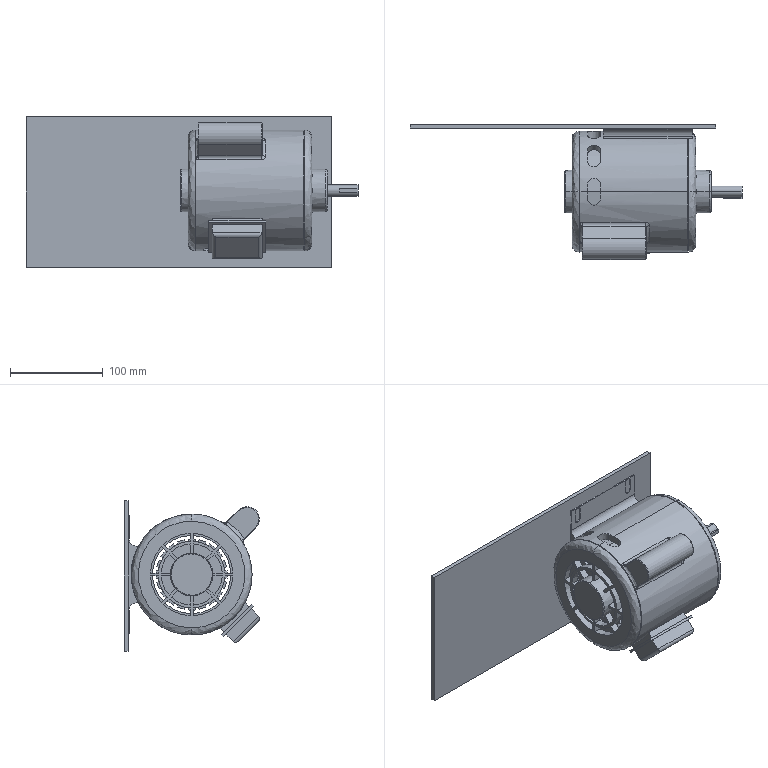Part | STEP file | _X2_51434EF6_X0_22_1 | 25 solids | 517 faces | box 358.567 x 145.946 x 163 mm | volume 1839939 mm3 | cylinder 220 | plane 219 | spline 70 | cone 8 | commonest cylinder face diameters 1.536 x53 69.12 x23 76.8 x21 13.824 x17 66.048 x16 72.192 x16